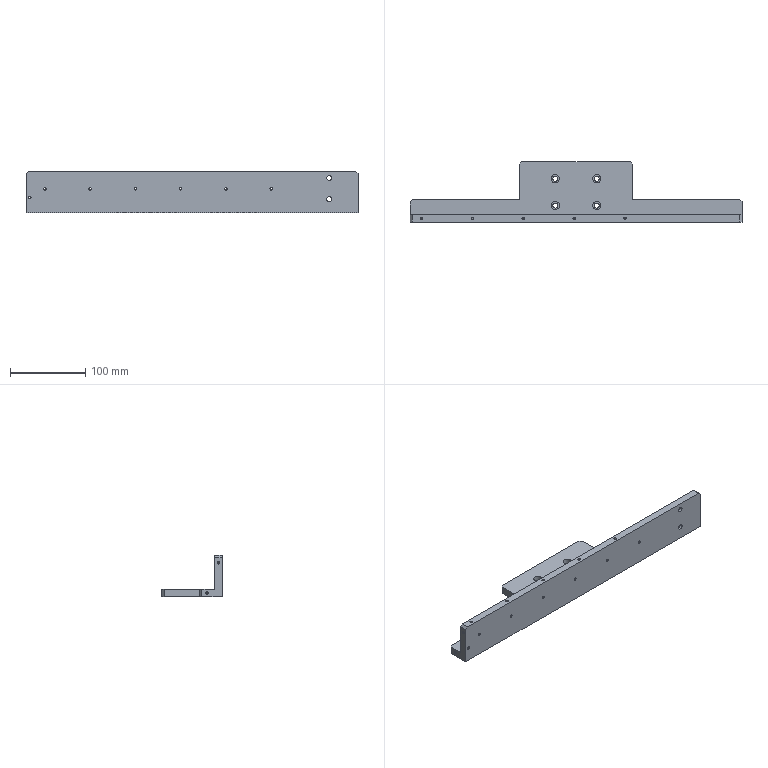Part | SolidWorks | features HoleWzd 7, ICE 2, Chamfer 1, Extrusion 1, MirrorPattern 1 | 1 solid | 106 faces | box 440 x 80 x 55 mm | volume 398630 mm3 | cylinder 60 | plane 24 | cone 22 | commonest cylinder face diameters 3.3 x36 6.6 x12 11 x12